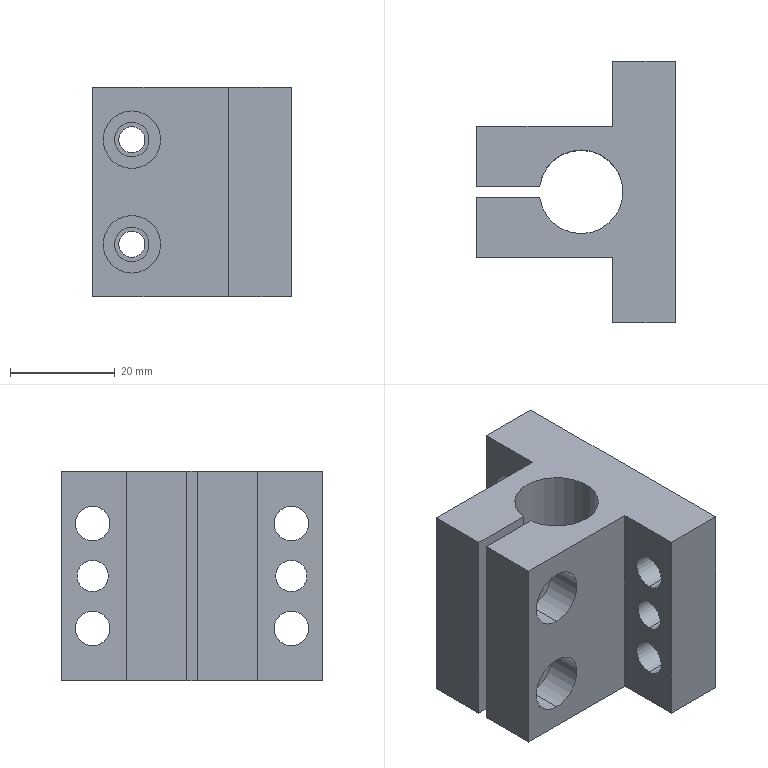Part | STEP file | CLPM16 | 1 solid | 40 faces | box 38 x 50 x 40 mm | volume 36609 mm3 | cylinder 25 | plane 15 | commonest cylinder face diameters 6.6 x12 5 x4 6 x4 11 x4 16 x1
STEP:
#1=CARTESIAN_POINT('',(18.,-19.,17.));
#2=VERTEX_POINT('',#1);
#3=CARTESIAN_POINT('',(18.,-19.,23.));
#4=VERTEX_POINT('',#3);
#5=CARTESIAN_POINT('',(18.,-19.,20.));
#6=DIRECTION('',(-1.,0.,0.));
#7=DIRECTION('',(0.,-1.,0.));
#8=AXIS2_PLACEMENT_3D('',#5,#6,#7);
#9=CIRCLE('',#8,3.);
#10=EDGE_CURVE('',#2,#4,#9,.T.);
#11=ORIENTED_EDGE('',*,*,#10,.F.);
#12=CARTESIAN_POINT('',(6.,-19.,17.));
#13=VERTEX_POINT('',#12);
#14=CARTESIAN_POINT('',(6.,-19.,17.));
#15=DIRECTION('',(-1.,0.,0.));
#16=VECTOR('',#15,1000.);
#17=LINE('',#14,#16);
#18=EDGE_CURVE('',#2,#13,#17,.T.);
#19=ORIENTED_EDGE('',*,*,#18,.T.);
#20=CARTESIAN_POINT('',(6.,-19.,23.));
#21=VERTEX_POINT('',#20);
#22=CARTESIAN_POINT('',(6.,-19.,20.));
#23=DIRECTION('',(-1.,0.,0.));
#24=DIRECTION('',(0.,0.,1.));
#25=AXIS2_PLACEMENT_3D('',#22,#23,#24);
#26=CIRCLE('',#25,3.);
#27=EDGE_CURVE('',#13,#21,#26,.T.);
#28=ORIENTED_EDGE('',*,*,#27,.T.);
#29=CARTESIAN_POINT('',(6.,-19.,23.));
#30=DIRECTION('',(-1.,0.,0.));
#31=VECTOR('',#30,1000.);
#32=LINE('',#29,#31);
#33=EDGE_CURVE('',#4,#21,#32,.T.);
#34=ORIENTED_EDGE('',*,*,#33,.F.);
#35=EDGE_LOOP('',(#11,#19,#28,#34));
#36=FACE_OUTER_BOUND('',#35,.T.);
#37=CARTESIAN_POINT('',(6.,-19.,20.));
#38=DIRECTION('',(-1.,0.,0.));
#39=DIRECTION('',(0.,0.,1.));
#40=AXIS2_PLACEMENT_3D('',#37,#38,#39);
#41=CYLINDRICAL_SURFACE('',#40,3.);
#42=ADVANCED_FACE('',(#36),#41,.F.);
#43=CARTESIAN_POINT('',(18.,19.,17.));
#44=VERTEX_POINT('',#43);
#45=CARTESIAN_POINT('',(18.,19.,23.));
#46=VERTEX_POINT('',#45);
#47=CARTESIAN_POINT('',(18.,19.,20.));
#48=DIRECTION('',(-1.,0.,0.));
#49=DIRECTION('',(0.,-1.,0.));
#50=AXIS2_PLACEMENT_3D('',#47,#48,#49);
#51=CIRCLE('',#50,3.);
#52=EDGE_CURVE('',#44,#46,#51,.T.);
#53=ORIENTED_EDGE('',*,*,#52,.F.);
#54=CARTESIAN_POINT('',(6.,19.,17.));
#55=VERTEX_POINT('',#54);
#56=CARTESIAN_POINT('',(6.,19.,17.));
#57=DIRECTION('',(-1.,0.,0.));
#58=VECTOR('',#57,1000.);
#59=LINE('',#56,#58);
#60=EDGE_CURVE('',#44,#55,#59,.T.);
#61=ORIENTED_EDGE('',*,*,#60,.T.);
#62=CARTESIAN_POINT('',(6.,19.,23.));
#63=VERTEX_POINT('',#62);
#64=CARTESIAN_POINT('',(6.,19.,20.));
#65=DIRECTION('',(-1.,0.,0.));
#66=DIRECTION('',(0.,0.,1.));
#67=AXIS2_PLACEMENT_3D('',#64,#65,#66);
#68=CIRCLE('',#67,3.);
#69=EDGE_CURVE('',#55,#63,#68,.T.);
#70=ORIENTED_EDGE('',*,*,#69,.T.);
#71=CARTESIAN_POINT('',(6.,19.,23.));
#72=DIRECTION('',(-1.,0.,0.));
#73=VECTOR('',#72,1000.);
#74=LINE('',#71,#73);
#75=EDGE_CURVE('',#46,#63,#74,.T.);
#76=ORIENTED_EDGE('',*,*,#75,.F.);
#77=EDGE_LOOP('',(#53,#61,#70,#76));
#78=FACE_OUTER_BOUND('',#77,.T.);
#79=CARTESIAN_POINT('',(6.,19.,20.));
#80=DIRECTION('',(-1.,0.,0.));
#81=DIRECTION('',(0.,0.,1.));
#82=AXIS2_PLACEMENT_3D('',#79,#80,#81);
#83=CYLINDRICAL_SURFACE('',#82,3.);
#84=ADVANCED_FACE('',(#78),#83,.F.);
#85=CARTESIAN_POINT('',(18.,19.,26.7));
#86=VERTEX_POINT('',#85);
#87=CARTESIAN_POINT('',(18.,19.,33.3));
#88=VERTEX_POINT('',#87);
#89=CARTESIAN_POINT('',(18.,19.,30.));
#90=DIRECTION('',(-1.,0.,0.));
#91=DIRECTION('',(0.,-1.,0.));
#92=AXIS2_PLACEMENT_3D('',#89,#90,#91);
#93=CIRCLE('',#92,3.3);
#94=EDGE_CURVE('',#86,#88,#93,.T.);
#95=ORIENTED_EDGE('',*,*,#94,.F.);
#96=CARTESIAN_POINT('',(6.,19.,26.7));
#97=VERTEX_POINT('',#96);
#98=CARTESIAN_POINT('',(6.,19.,26.7));
#99=DIRECTION('',(-1.,0.,0.));
#100=VECTOR('',#99,1000.);
#101=LINE('',#98,#100);
#102=EDGE_CURVE('',#86,#97,#101,.T.);
#103=ORIENTED_EDGE('',*,*,#102,.T.);
#104=CARTESIAN_POINT('',(6.,19.,33.3));
#105=VERTEX_POINT('',#104);
#106=CARTESIAN_POINT('',(6.,19.,30.));
#107=DIRECTION('',(-1.,0.,0.));
#108=DIRECTION('',(0.,0.,1.));
#109=AXIS2_PLACEMENT_3D('',#106,#107,#108);
#110=CIRCLE('',#109,3.3);
#111=EDGE_CURVE('',#97,#105,#110,.T.);
#112=ORIENTED_EDGE('',*,*,#111,.T.);
#113=CARTESIAN_POINT('',(6.,19.,33.3));
#114=DIRECTION('',(-1.,0.,0.));
#115=VECTOR('',#114,1000.);
#116=LINE('',#113,#115);
#117=EDGE_CURVE('',#88,#105,#116,.T.);
#118=ORIENTED_EDGE('',*,*,#117,.F.);
#119=EDGE_LOOP('',(#95,#103,#112,#118));
#120=FACE_OUTER_BOUND('',#119,.T.);
#121=CARTESIAN_POINT('',(6.,19.,30.));
#122=DIRECTION('',(-1.,0.,0.));
#123=DIRECTION('',(0.,0.,1.));
#124=AXIS2_PLACEMENT_3D('',#121,#122,#123);
#125=CYLINDRICAL_SURFACE('',#124,3.3);
#126=ADVANCED_FACE('',(#120),#125,.F.);
#127=CARTESIAN_POINT('',(18.,19.,6.7));
#128=VERTEX_POINT('',#127);
#129=CARTESIAN_POINT('',(18.,19.,13.3));
#130=VERTEX_POINT('',#129);
#131=CARTESIAN_POINT('',(18.,19.,10.));
#132=DIRECTION('',(-1.,0.,0.));
#133=DIRECTION('',(0.,-1.,0.));
#134=AXIS2_PLACEMENT_3D('',#131,#132,#133);
#135=CIRCLE('',#134,3.3);
#136=EDGE_CURVE('',#128,#130,#135,.T.);
#137=ORIENTED_EDGE('',*,*,#136,.F.);
#138=CARTESIAN_POINT('',(6.,19.,6.7));
#139=VERTEX_POINT('',#138);
#140=CARTESIAN_POINT('',(6.,19.,6.7));
#141=DIRECTION('',(-1.,0.,0.));
#142=VECTOR('',#141,1000.);
#143=LINE('',#140,#142);
#144=EDGE_CURVE('',#128,#139,#143,.T.);
#145=ORIENTED_EDGE('',*,*,#144,.T.);
#146=CARTESIAN_POINT('',(6.,19.,13.3));
#147=VERTEX_POINT('',#146);
#148=CARTESIAN_POINT('',(6.,19.,10.));
#149=DIRECTION('',(-1.,0.,0.));
#150=DIRECTION('',(0.,0.,1.));
#151=AXIS2_PLACEMENT_3D('',#148,#149,#150);
#152=CIRCLE('',#151,3.3);
#153=EDGE_CURVE('',#139,#147,#152,.T.);
#154=ORIENTED_EDGE('',*,*,#153,.T.);
#155=CARTESIAN_POINT('',(6.,19.,13.3));
#156=DIRECTION('',(-1.,0.,0.));
#157=VECTOR('',#156,1000.);
#158=LINE('',#155,#157);
#159=EDGE_CURVE('',#130,#147,#158,.T.);
#160=ORIENTED_EDGE('',*,*,#159,.F.);
#161=EDGE_LOOP('',(#137,#145,#154,#160));
#162=FACE_OUTER_BOUND('',#161,.T.);
#163=CARTESIAN_POINT('',(6.,19.,10.));
#164=DIRECTION('',(-1.,0.,0.));
#165=DIRECTION('',(0.,0.,1.));
#166=AXIS2_PLACEMENT_3D('',#163,#164,#165);
#167=CYLINDRICAL_SURFACE('',#166,3.3);
#168=ADVANCED_FACE('',(#162),#167,.F.);
#169=CARTESIAN_POINT('',(18.,-19.,6.7));
#170=VERTEX_POINT('',#169);
#171=CARTESIAN_POINT('',(18.,-19.,13.3));
#172=VERTEX_POINT('',#171);
#173=CARTESIAN_POINT('',(18.,-19.,10.));
#174=DIRECTION('',(-1.,0.,0.));
#175=DIRECTION('',(0.,-1.,0.));
#176=AXIS2_PLACEMENT_3D('',#173,#174,#175);
#177=CIRCLE('',#176,3.3);
#178=EDGE_CURVE('',#170,#172,#177,.T.);
#179=ORIENTED_EDGE('',*,*,#178,.F.);
#180=CARTESIAN_POINT('',(6.,-19.,6.7));
#181=VERTEX_POINT('',#180);
#182=CARTESIAN_POINT('',(6.,-19.,6.7));
#183=DIRECTION('',(-1.,0.,0.));
#184=VECTOR('',#183,1000.);
#185=LINE('',#182,#184);
#186=EDGE_CURVE('',#170,#181,#185,.T.);
#187=ORIENTED_EDGE('',*,*,#186,.T.);
#188=CARTESIAN_POINT('',(6.,-19.,13.3));
#189=VERTEX_POINT('',#188);
#190=CARTESIAN_POINT('',(6.,-19.,10.));
#191=DIRECTION('',(-1.,0.,0.));
#192=DIRECTION('',(0.,0.,1.));
#193=AXIS2_PLACEMENT_3D('',#190,#191,#192);
#194=CIRCLE('',#193,3.3);
#195=EDGE_CURVE('',#181,#189,#194,.T.);
#196=ORIENTED_EDGE('',*,*,#195,.T.);
#197=CARTESIAN_POINT('',(6.,-19.,13.3));
#198=DIRECTION('',(-1.,0.,0.));
#199=VECTOR('',#198,1000.);
#200=LINE('',#197,#199);
#201=EDGE_CURVE('',#172,#189,#200,.T.);
#202=ORIENTED_EDGE('',*,*,#201,.F.);
#203=EDGE_LOOP('',(#179,#187,#196,#202));
#204=FACE_OUTER_BOUND('',#203,.T.);
#205=CARTESIAN_POINT('',(6.,-19.,10.));
#206=DIRECTION('',(-1.,0.,0.));
#207=DIRECTION('',(0.,0.,1.));
#208=AXIS2_PLACEMENT_3D('',#205,#206,#207);
#209=CYLINDRICAL_SURFACE('',#208,3.3);
#210=ADVANCED_FACE('',(#204),#209,.F.);
#211=CARTESIAN_POINT('',(18.,-19.,26.7));
#212=VERTEX_POINT('',#211);
#213=CARTESIAN_POINT('',(18.,-19.,33.3));
#214=VERTEX_POINT('',#213);
#215=CARTESIAN_POINT('',(18.,-19.,30.));
#216=DIRECTION('',(-1.,0.,0.));
#217=DIRECTION('',(0.,-1.,0.));
#218=AXIS2_PLACEMENT_3D('',#215,#216,#217);
#219=CIRCLE('',#218,3.3);
#220=EDGE_CURVE('',#212,#214,#219,.T.);
#221=ORIENTED_EDGE('',*,*,#220,.F.);
#222=CARTESIAN_POINT('',(6.,-19.,26.7));
#223=VERTEX_POINT('',#222);
#224=CARTESIAN_POINT('',(6.,-19.,26.7));
#225=DIRECTION('',(-1.,0.,0.));
#226=VECTOR('',#225,1000.);
#227=LINE('',#224,#226);
#228=EDGE_CURVE('',#212,#223,#227,.T.);
#229=ORIENTED_EDGE('',*,*,#228,.T.);
#230=CARTESIAN_POINT('',(6.,-19.,33.3));
#231=VERTEX_POINT('',#230);
#232=CARTESIAN_POINT('',(6.,-19.,30.));
#233=DIRECTION('',(-1.,0.,0.));
#234=DIRECTION('',(0.,0.,1.));
#235=AXIS2_PLACEMENT_3D('',#232,#233,#234);
#236=CIRCLE('',#235,3.3);
#237=EDGE_CURVE('',#223,#231,#236,.T.);
#238=ORIENTED_EDGE('',*,*,#237,.T.);
#239=CARTESIAN_POINT('',(6.,-19.,33.3));
#240=DIRECTION('',(-1.,0.,0.));
#241=VECTOR('',#240,1000.);
#242=LINE('',#239,#241);
#243=EDGE_CURVE('',#214,#231,#242,.T.);
#244=ORIENTED_EDGE('',*,*,#243,.F.);
#245=EDGE_LOOP('',(#221,#229,#238,#244));
#246=FACE_OUTER_BOUND('',#245,.T.);
#247=CARTESIAN_POINT('',(6.,-19.,30.));
#248=DIRECTION('',(-1.,0.,0.));
#249=DIRECTION('',(0.,0.,1.));
#250=AXIS2_PLACEMENT_3D('',#247,#248,#249);
#251=CYLINDRICAL_SURFACE('',#250,3.3);
#252=ADVANCED_FACE('',(#246),#251,.F.);
#253=CARTESIAN_POINT('',(-12.5,12.5,12.5));
#254=VERTEX_POINT('',#253);
#255=CARTESIAN_POINT('',(-12.5,12.5,7.5));
#256=VERTEX_POINT('',#255);
#257=CARTESIAN_POINT('',(-12.5,12.5,10.));
#258=DIRECTION('',(0.,-1.,0.));
#259=DIRECTION('',(0.,0.,-1.));
#260=AXIS2_PLACEMENT_3D('',#257,#258,#259);
#261=CIRCLE('',#260,2.5);
#262=EDGE_CURVE('',#254,#256,#261,.T.);
#263=ORIENTED_EDGE('',*,*,#262,.F.);
#264=CARTESIAN_POINT('',(-12.5,1.,12.5));
#265=VERTEX_POINT('',#264);
#266=CARTESIAN_POINT('',(-12.5,1.,12.5));
#267=DIRECTION('',(0.,-1.,0.));
#268=VECTOR('',#267,1000.);
#269=LINE('',#266,#268);
#270=EDGE_CURVE('',#254,#265,#269,.T.);
#271=ORIENTED_EDGE('',*,*,#270,.T.);
#272=CARTESIAN_POINT('',(-12.5,1.,7.5));
#273=VERTEX_POINT('',#272);
#274=CARTESIAN_POINT('',(-12.5,1.,10.));
#275=DIRECTION('',(0.,-1.,0.));
#276=DIRECTION('',(0.,0.,-1.));
#277=AXIS2_PLACEMENT_3D('',#274,#275,#276);
#278=CIRCLE('',#277,2.5);
#279=EDGE_CURVE('',#265,#273,#278,.T.);
#280=ORIENTED_EDGE('',*,*,#279,.T.);
#281=CARTESIAN_POINT('',(-12.5,1.,7.5));
#282=DIRECTION('',(0.,-1.,0.));
#283=VECTOR('',#282,1000.);
#284=LINE('',#281,#283);
#285=EDGE_CURVE('',#256,#273,#284,.T.);
#286=ORIENTED_EDGE('',*,*,#285,.F.);
#287=EDGE_LOOP('',(#263,#271,#280,#286));
#288=FACE_OUTER_BOUND('',#287,.T.);
#289=CARTESIAN_POINT('',(-12.5,1.,10.));
#290=DIRECTION('',(0.,-1.,0.));
#291=DIRECTION('',(0.,0.,-1.));
#292=AXIS2_PLACEMENT_3D('',#289,#290,#291);
#293=CYLINDRICAL_SURFACE('',#292,2.5);
#294=ADVANCED_FACE('',(#288),#293,.F.);
#295=CARTESIAN_POINT('',(-12.5,12.5,32.5));
#296=VERTEX_POINT('',#295);
#297=CARTESIAN_POINT('',(-12.5,12.5,27.5));
#298=VERTEX_POINT('',#297);
#299=CARTESIAN_POINT('',(-12.5,12.5,30.));
#300=DIRECTION('',(0.,-1.,0.));
#301=DIRECTION('',(0.,0.,-1.));
#302=AXIS2_PLACEMENT_3D('',#299,#300,#301);
#303=CIRCLE('',#302,2.5);
#304=EDGE_CURVE('',#296,#298,#303,.T.);
#305=ORIENTED_EDGE('',*,*,#304,.F.);
#306=CARTESIAN_POINT('',(-12.5,1.,32.5));
#307=VERTEX_POINT('',#306);
#308=CARTESIAN_POINT('',(-12.5,1.,32.5));
#309=DIRECTION('',(0.,-1.,0.));
#310=VECTOR('',#309,1000.);
#311=LINE('',#308,#310);
#312=EDGE_CURVE('',#296,#307,#311,.T.);
#313=ORIENTED_EDGE('',*,*,#312,.T.);
#314=CARTESIAN_POINT('',(-12.5,1.,27.5));
#315=VERTEX_POINT('',#314);
#316=CARTESIAN_POINT('',(-12.5,1.,30.));
#317=DIRECTION('',(0.,-1.,0.));
#318=DIRECTION('',(0.,0.,-1.));
#319=AXIS2_PLACEMENT_3D('',#316,#317,#318);
#320=CIRCLE('',#319,2.5);
#321=EDGE_CURVE('',#307,#315,#320,.T.);
#322=ORIENTED_EDGE('',*,*,#321,.T.);
#323=CARTESIAN_POINT('',(-12.5,1.,27.5));
#324=DIRECTION('',(0.,-1.,0.));
#325=VECTOR('',#324,1000.);
#326=LINE('',#323,#325);
#327=EDGE_CURVE('',#298,#315,#326,.T.);
#328=ORIENTED_EDGE('',*,*,#327,.F.);
#329=EDGE_LOOP('',(#305,#313,#322,#328));
#330=FACE_OUTER_BOUND('',#329,.T.);
#331=CARTESIAN_POINT('',(-12.5,1.,30.));
#332=DIRECTION('',(0.,-1.,0.));
#333=DIRECTION('',(0.,0.,-1.));
#334=AXIS2_PLACEMENT_3D('',#331,#332,#333);
#335=CYLINDRICAL_SURFACE('',#334,2.5);
#336=ADVANCED_FACE('',(#330),#335,.F.);
#337=CARTESIAN_POINT('',(-12.5,-5.7,15.5));
#338=VERTEX_POINT('',#337);
#339=CARTESIAN_POINT('',(-12.5,-5.7,4.5));
#340=VERTEX_POINT('',#339);
#341=CARTESIAN_POINT('',(-12.5,-5.7,10.));
#342=DIRECTION('',(0.,-1.,0.));
#343=DIRECTION('',(0.,0.,-1.));
#344=AXIS2_PLACEMENT_3D('',#341,#342,#343);
#345=CIRCLE('',#344,5.5);
#346=EDGE_CURVE('',#338,#340,#345,.T.);
#347=ORIENTED_EDGE('',*,*,#346,.F.);
#348=CARTESIAN_POINT('',(-12.5,-12.5,15.5));
#349=VERTEX_POINT('',#348);
#350=CARTESIAN_POINT('',(-12.5,-12.5,15.5));
#351=DIRECTION('',(0.,-1.,0.));
#352=VECTOR('',#351,1000.);
#353=LINE('',#350,#352);
#354=EDGE_CURVE('',#338,#349,#353,.T.);
#355=ORIENTED_EDGE('',*,*,#354,.T.);
#356=CARTESIAN_POINT('',(-12.5,-12.5,4.5));
#357=VERTEX_POINT('',#356);
#358=CARTESIAN_POINT('',(-12.5,-12.5,10.));
#359=DIRECTION('',(0.,-1.,0.));
#360=DIRECTION('',(0.,0.,-1.));
#361=AXIS2_PLACEMENT_3D('',#358,#359,#360);
#362=CIRCLE('',#361,5.5);
#363=EDGE_CURVE('',#349,#357,#362,.T.);
#364=ORIENTED_EDGE('',*,*,#363,.T.);
#365=CARTESIAN_POINT('',(-12.5,-12.5,4.5));
#366=DIRECTION('',(0.,-1.,0.));
#367=VECTOR('',#366,1000.);
#368=LINE('',#365,#367);
#369=EDGE_CURVE('',#340,#357,#368,.T.);
#370=ORIENTED_EDGE('',*,*,#369,.F.);
#371=EDGE_LOOP('',(#347,#355,#364,#370));
#372=FACE_OUTER_BOUND('',#371,.T.);
#373=CARTESIAN_POINT('',(-12.5,-12.5,10.));
#374=DIRECTION('',(0.,-1.,0.));
#375=DIRECTION('',(0.,0.,-1.));
#376=AXIS2_PLACEMENT_3D('',#373,#374,#375);
#377=CYLINDRICAL_SURFACE('',#376,5.5);
#378=ADVANCED_FACE('',(#372),#377,.F.);
#379=CARTESIAN_POINT('',(-12.5,-1.,13.3));
#380=VERTEX_POINT('',#379);
#381=CARTESIAN_POINT('',(-12.5,-1.,6.7));
#382=VERTEX_POINT('',#381);
#383=CARTESIAN_POINT('',(-12.5,-1.,10.));
#384=DIRECTION('',(0.,-1.,0.));
#385=DIRECTION('',(1.,0.,0.));
#386=AXIS2_PLACEMENT_3D('',#383,#384,#385);
#387=CIRCLE('',#386,3.3);
#388=EDGE_CURVE('',#380,#382,#387,.T.);
#389=ORIENTED_EDGE('',*,*,#388,.F.);
#390=CARTESIAN_POINT('',(-12.5,-5.7,13.3));
#391=VERTEX_POINT('',#390);
#392=CARTESIAN_POINT('',(-12.5,-12.5,13.3));
#393=DIRECTION('',(0.,-1.,0.));
#394=VECTOR('',#393,1000.);
#395=LINE('',#392,#394);
#396=EDGE_CURVE('',#380,#391,#395,.T.);
#397=ORIENTED_EDGE('',*,*,#396,.T.);
#398=CARTESIAN_POINT('',(-12.5,-5.7,6.7));
#399=VERTEX_POINT('',#398);
#400=CARTESIAN_POINT('',(-12.5,-5.7,10.));
#401=DIRECTION('',(0.,-1.,0.));
#402=DIRECTION('',(0.,0.,-1.));
#403=AXIS2_PLACEMENT_3D('',#400,#401,#402);
#404=CIRCLE('',#403,3.3);
#405=EDGE_CURVE('',#391,#399,#404,.T.);
#406=ORIENTED_EDGE('',*,*,#405,.T.);
#407=CARTESIAN_POINT('',(-12.5,-12.5,6.7));
#408=DIRECTION('',(0.,-1.,0.));
#409=VECTOR('',#408,1000.);
#410=LINE('',#407,#409);
#411=EDGE_CURVE('',#382,#399,#410,.T.);
#412=ORIENTED_EDGE('',*,*,#411,.F.);
#413=EDGE_LOOP('',(#389,#397,#406,#412));
#414=FACE_OUTER_BOUND('',#413,.T.);
#415=CARTESIAN_POINT('',(-12.5,-12.5,10.));
#416=DIRECTION('',(0.,-1.,0.));
#417=DIRECTION('',(0.,0.,-1.));
#418=AXIS2_PLACEMENT_3D('',#415,#416,#417);
#419=CYLINDRICAL_SURFACE('',#418,3.3);
#420=ADVANCED_FACE('',(#414),#419,.F.);
#421=CARTESIAN_POINT('',(-12.5,-5.7,35.5));
#422=VERTEX_POINT('',#421);
#423=CARTESIAN_POINT('',(-12.5,-5.7,24.5));
#424=VERTEX_POINT('',#423);
#425=CARTESIAN_POINT('',(-12.5,-5.7,30.));
#426=DIRECTION('',(0.,-1.,0.));
#427=DIRECTION('',(0.,0.,-1.));
#428=AXIS2_PLACEMENT_3D('',#425,#426,#427);
#429=CIRCLE('',#428,5.5);
#430=EDGE_CURVE('',#422,#424,#429,.T.);
#431=ORIENTED_EDGE('',*,*,#430,.F.);
#432=CARTESIAN_POINT('',(-12.5,-12.5,35.5));
#433=VERTEX_POINT('',#432);
#434=CARTESIAN_POINT('',(-12.5,-12.5,35.5));
#435=DIRECTION('',(0.,-1.,0.));
#436=VECTOR('',#435,1000.);
#437=LINE('',#434,#436);
#438=EDGE_CURVE('',#422,#433,#437,.T.);
#439=ORIENTED_EDGE('',*,*,#438,.T.);
#440=CARTESIAN_POINT('',(-12.5,-12.5,24.5));
#441=VERTEX_POINT('',#440);
#442=CARTESIAN_POINT('',(-12.5,-12.5,30.));
#443=DIRECTION('',(0.,-1.,0.));
#444=DIRECTION('',(0.,0.,-1.));
#445=AXIS2_PLACEMENT_3D('',#442,#443,#444);
#446=CIRCLE('',#445,5.5);
#447=EDGE_CURVE('',#433,#441,#446,.T.);
#448=ORIENTED_EDGE('',*,*,#447,.T.);
#449=CARTESIAN_POINT('',(-12.5,-12.5,24.5));
#450=DIRECTION('',(0.,-1.,0.));
#451=VECTOR('',#450,1000.);
#452=LINE('',#449,#451);
#453=EDGE_CURVE('',#424,#441,#452,.T.);
#454=ORIENTED_EDGE('',*,*,#453,.F.);
#455=EDGE_LOOP('',(#431,#439,#448,#454));
#456=FACE_OUTER_BOUND('',#455,.T.);
#457=CARTESIAN_POINT('',(-12.5,-12.5,30.));
#458=DIRECTION('',(0.,-1.,0.));
#459=DIRECTION('',(0.,0.,-1.));
#460=AXIS2_PLACEMENT_3D('',#457,#458,#459);
#461=CYLINDRICAL_SURFACE('',#460,5.5);
#462=ADVANCED_FACE('',(#456),#461,.F.);
#463=CARTESIAN_POINT('',(-12.5,-1.,33.3));
#464=VERTEX_POINT('',#463);
#465=CARTESIAN_POINT('',(-12.5,-1.,26.7));
#466=VERTEX_POINT('',#465);
#467=CARTESIAN_POINT('',(-12.5,-1.,30.));
#468=DIRECTION('',(0.,-1.,0.));
#469=DIRECTION('',(1.,0.,0.));
#470=AXIS2_PLACEMENT_3D('',#467,#468,#469);
#471=CIRCLE('',#470,3.3);
#472=EDGE_CURVE('',#464,#466,#471,.T.);
#473=ORIENTED_EDGE('',*,*,#472,.F.);
#474=CARTESIAN_POINT('',(-12.5,-5.7,33.3));
#475=VERTEX_POINT('',#474);
#476=CARTESIAN_POINT('',(-12.5,-12.5,33.3));
#477=DIRECTION('',(0.,-1.,0.));
#478=VECTOR('',#477,1000.);
#479=LINE('',#476,#478);
#480=EDGE_CURVE('',#464,#475,#479,.T.);
#481=ORIENTED_EDGE('',*,*,#480,.T.);
#482=CARTESIAN_POINT('',(-12.5,-5.7,26.7));
#483=VERTEX_POINT('',#482);
#484=CARTESIAN_POINT('',(-12.5,-5.7,30.));
#485=DIRECTION('',(0.,-1.,0.));
#486=DIRECTION('',(0.,0.,-1.));
#487=AXIS2_PLACEMENT_3D('',#484,#485,#486);
#488=CIRCLE('',#487,3.3);
#489=EDGE_CURVE('',#475,#483,#488,.T.);
#490=ORIENTED_EDGE('',*,*,#489,.T.);
#491=CARTESIAN_POINT('',(-12.5,-12.5,26.7));
#492=DIRECTION('',(0.,-1.,0.));
#493=VECTOR('',#492,1000.);
#494=LINE('',#491,#493);
#495=EDGE_CURVE('',#466,#483,#494,.T.);
#496=ORIENTED_EDGE('',*,*,#495,.F.);
#497=EDGE_LOOP('',(#473,#481,#490,#496));
#498=FACE_OUTER_BOUND('',#497,.T.);
#499=CARTESIAN_POINT('',(-12.5,-12.5,30.));
#500=DIRECTION('',(0.,-1.,0.));
#501=DIRECTION('',(0.,0.,-1.));
#502=AXIS2_PLACEMENT_3D('',#499,#500,#501);
#503=CYLINDRICAL_SURFACE('',#502,3.3);
#504=ADVANCED_FACE('',(#498),#503,.F.);
#505=CARTESIAN_POINT('',(-12.5,-12.5,30.));
#506=DIRECTION('',(0.,-1.,0.));
#507=DIRECTION('',(0.,0.,-1.));
#508=AXIS2_PLACEMENT_3D('',#505,#506,#507);
#509=CIRCLE('',#508,5.5);
#510=EDGE_CURVE('',#441,#433,#509,.T.);
#511=ORIENTED_EDGE('',*,*,#510,.F.);
#512=ORIENTED_EDGE('',*,*,#447,.F.);
#513=EDGE_LOOP('',(#511,#512));
#514=FACE_BOUND('',#513,.T.);
#515=CARTESIAN_POINT('',(-20.,-12.5,0.));
#516=VERTEX_POINT('',#515);
#517=CARTESIAN_POINT('',(6.,-12.5,0.));
#518=VERTEX_POINT('',#517);
#519=CARTESIAN_POINT('',(-20.,-12.5,0.));
#520=DIRECTION('',(1.,0.,0.));
#521=VECTOR('',#520,1000.);
#522=LINE('',#519,#521);
#523=EDGE_CURVE('',#516,#518,#522,.T.);
#524=ORIENTED_EDGE('',*,*,#523,.T.);
#525=CARTESIAN_POINT('',(6.,-12.5,40.));
#526=VERTEX_POINT('',#525);
#527=CARTESIAN_POINT('',(6.,-12.5,40.));
#528=DIRECTION('',(0.,0.,-1.));
#529=VECTOR('',#528,1000.);
#530=LINE('',#527,#529);
#531=EDGE_CURVE('',#526,#518,#530,.T.);
#532=ORIENTED_EDGE('',*,*,#531,.F.);
#533=CARTESIAN_POINT('',(-20.,-12.5,40.));
#534=VERTEX_POINT('',#533);
#535=CARTESIAN_POINT('',(-20.,-12.5,40.));
#536=DIRECTION('',(1.,0.,0.));
#537=VECTOR('',#536,1000.);
#538=LINE('',#535,#537);
#539=EDGE_CURVE('',#534,#526,#538,.T.);
#540=ORIENTED_EDGE('',*,*,#539,.F.);
#541=CARTESIAN_POINT('',(-20.,-12.5,40.));
#542=DIRECTION('',(0.,0.,-1.));
#543=VECTOR('',#542,1000.);
#544=LINE('',#541,#543);
#545=EDGE_CURVE('',#534,#516,#544,.T.);
#546=ORIENTED_EDGE('',*,*,#545,.T.);
#547=EDGE_LOOP('',(#524,#532,#540,#546));
#548=FACE_OUTER_BOUND('',#547,.T.);
#549=CARTESIAN_POINT('',(-12.5,-12.5,10.));
#550=DIRECTION('',(0.,-1.,0.));
#551=DIRECTION('',(0.,0.,-1.));
#552=AXIS2_PLACEMENT_3D('',#549,#550,#551);
#553=CIRCLE('',#552,5.5);
#554=EDGE_CURVE('',#357,#349,#553,.T.);
#555=ORIENTED_EDGE('',*,*,#554,.F.);
#556=ORIENTED_EDGE('',*,*,#363,.F.);
#557=EDGE_LOOP('',(#555,#556));
#558=FACE_BOUND('',#557,.T.);
#559=CARTESIAN_POINT('',(-20.,-12.5,40.));
#560=DIRECTION('',(0.,1.,0.));
#561=DIRECTION('',(0.,0.,1.));
#562=AXIS2_PLACEMENT_3D('',#559,#560,#561);
#563=PLANE('',#562);
#564=ADVANCED_FACE('',(#514,#548,#558),#563,.F.);
#565=CARTESIAN_POINT('',(-20.,-1.,0.));
#566=VERTEX_POINT('',#565);
#567=CARTESIAN_POINT('',(-20.,-1.,0.));
#568=DIRECTION('',(0.,-1.,0.));
#569=VECTOR('',#568,1000.);
#570=LINE('',#567,#569);
#571=EDGE_CURVE('',#566,#516,#570,.T.);
#572=ORIENTED_EDGE('',*,*,#571,.T.);
#573=ORIENTED_EDGE('',*,*,#545,.F.);
#574=CARTESIAN_POINT('',(-20.,-1.,40.));
#575=VERTEX_POINT('',#574);
#576=CARTESIAN_POINT('',(-20.,-1.,40.));
#577=DIRECTION('',(0.,-1.,0.));
#578=VECTOR('',#577,1000.);
#579=LINE('',#576,#578);
#580=EDGE_CURVE('',#575,#534,#579,.T.);
#581=ORIENTED_EDGE('',*,*,#580,.F.);
#582=CARTESIAN_POINT('',(-20.,-1.,40.));
#583=DIRECTION('',(0.,0.,-1.));
#584=VECTOR('',#583,1000.);
#585=LINE('',#582,#584);
#586=EDGE_CURVE('',#575,#566,#585,.T.);
#587=ORIENTED_EDGE('',*,*,#586,.T.);
#588=EDGE_LOOP('',(#572,#573,#581,#587));
#589=FACE_OUTER_BOUND('',#588,.T.);
#590=CARTESIAN_POINT('',(-20.,-1.,40.));
#591=DIRECTION('',(1.,0.,0.));
#592=DIRECTION('',(0.,1.,0.));
#593=AXIS2_PLACEMENT_3D('',#590,#591,#592);
#594=PLANE('',#593);
#595=ADVANCED_FACE('',(#589),#594,.F.);
#596=CARTESIAN_POINT('',(6.,-19.,20.));
#597=DIRECTION('',(-1.,0.,0.));
#598=DIRECTION('',(0.,0.,1.));
#599=AXIS2_PLACEMENT_3D('',#596,#597,#598);
#600=CIRCLE('',#599,3.);
#601=EDGE_CURVE('',#21,#13,#600,.T.);
#602=ORIENTED_EDGE('',*,*,#601,.F.);
#603=ORIENTED_EDGE('',*,*,#27,.F.);
#604=EDGE_LOOP('',(#602,#603));
#605=FACE_BOUND('',#604,.T.);
#606=CARTESIAN_POINT('',(6.,-19.,10.));
#607=DIRECTION('',(-1.,0.,0.));
#608=DIRECTION('',(0.,0.,1.));
#609=AXIS2_PLACEMENT_3D('',#606,#607,#608);
#610=CIRCLE('',#609,3.3);
#611=EDGE_CURVE('',#189,#181,#610,.T.);
#612=ORIENTED_EDGE('',*,*,#611,.F.);
#613=ORIENTED_EDGE('',*,*,#195,.F.);
#614=EDGE_LOOP('',(#612,#613));
#615=FACE_BOUND('',#614,.T.);
#616=CARTESIAN_POINT('',(6.,-19.,30.));
#617=DIRECTION('',(-1.,0.,0.));
#618=DIRECTION('',(0.,0.,1.));
#619=AXIS2_PLACEMENT_3D('',#616,#617,#618);
#620=CIRCLE('',#619,3.3);
#621=EDGE_CURVE('',#231,#223,#620,.T.);
#622=ORIENTED_EDGE('',*,*,#621,.F.);
#623=ORIENTED_EDGE('',*,*,#237,.F.);
#624=EDGE_LOOP('',(#622,#623));
#625=FACE_BOUND('',#624,.T.);
#626=CARTESIAN_POINT('',(6.,-25.,0.));
#627=VERTEX_POINT('',#626);
#628=CARTESIAN_POINT('',(6.,-12.5,0.));
#629=DIRECTION('',(0.,-1.,0.));
#630=VECTOR('',#629,1000.);
#631=LINE('',#628,#630);
#632=EDGE_CURVE('',#518,#627,#631,.T.);
#633=ORIENTED_EDGE('',*,*,#632,.T.);
#634=CARTESIAN_POINT('',(6.,-25.,40.));
#635=VERTEX_POINT('',#634);
#636=CARTESIAN_POINT('',(6.,-25.,40.));
#637=DIRECTION('',(0.,0.,-1.));
#638=VECTOR('',#637,1000.);
#639=LINE('',#636,#638);
#640=EDGE_CURVE('',#635,#627,#639,.T.);
#641=ORIENTED_EDGE('',*,*,#640,.F.);
#642=CARTESIAN_POINT('',(6.,-12.5,40.));
#643=DIRECTION('',(0.,-1.,0.));
#644=VECTOR('',#643,1000.);
#645=LINE('',#642,#644);
#646=EDGE_CURVE('',#526,#635,#645,.T.);
#647=ORIENTED_EDGE('',*,*,#646,.F.);
#648=ORIENTED_EDGE('',*,*,#531,.T.);
#649=EDGE_LOOP('',(#633,#641,#647,#648));
#650=FACE_OUTER_BOUND('',#649,.T.);
#651=CARTESIAN_POINT('',(6.,-12.5,40.));
#652=DIRECTION('',(1.,0.,0.));
#653=DIRECTION('',(0.,1.,0.));
#654=AXIS2_PLACEMENT_3D('',#651,#652,#653);
#655=PLANE('',#654);
#656=ADVANCED_FACE('',(#605,#615,#625,#650),#655,.F.);
#657=CARTESIAN_POINT('',(18.,-25.,0.));
#658=VERTEX_POINT('',#657);
#659=CARTESIAN_POINT('',(6.,-25.,0.));
#660=DIRECTION('',(1.,0.,0.));
#661=VECTOR('',#660,1000.);
#662=LINE('',#659,#661);
#663=EDGE_CURVE('',#627,#658,#662,.T.);
#664=ORIENTED_EDGE('',*,*,#663,.T.);
#665=CARTESIAN_POINT('',(18.,-25.,40.));
#666=VERTEX_POINT('',#665);
#667=CARTESIAN_POINT('',(18.,-25.,40.));
#668=DIRECTION('',(0.,0.,-1.));
#669=VECTOR('',#668,1000.);
#670=LINE('',#667,#669);
#671=EDGE_CURVE('',#666,#658,#670,.T.);
#672=ORIENTED_EDGE('',*,*,#671,.F.);
#673=CARTESIAN_POINT('',(6.,-25.,40.));
#674=DIRECTION('',(1.,0.,0.));
#675=VECTOR('',#674,1000.);
#676=LINE('',#673,#675);
#677=EDGE_CURVE('',#635,#666,#676,.T.);
#678=ORIENTED_EDGE('',*,*,#677,.F.);
#679=ORIENTED_EDGE('',*,*,#640,.T.);
#680=EDGE_LOOP('',(#664,#672,#678,#679));
#681=FACE_OUTER_BOUND('',#680,.T.);
#682=CARTESIAN_POINT('',(6.,-25.,40.));
#683=DIRECTION('',(0.,1.,0.));
#684=DIRECTION('',(0.,0.,1.));
#685=AXIS2_PLACEMENT_3D('',#682,#683,#684);
#686=PLANE('',#685);
#687=ADVANCED_FACE('',(#681),#686,.F.);
#688=CARTESIAN_POINT('',(18.,-19.,20.));
#689=DIRECTION('',(-1.,0.,0.));
#690=DIRECTION('',(0.,-1.,0.));
#691=AXIS2_PLACEMENT_3D('',#688,#689,#690);
#692=CIRCLE('',#691,3.);
#693=EDGE_CURVE('',#4,#2,#692,.T.);
#694=ORIENTED_EDGE('',*,*,#693,.T.);
#695=ORIENTED_EDGE('',*,*,#10,.T.);
#696=EDGE_LOOP('',(#694,#695));
#697=FACE_BOUND('',#696,.T.);
#698=CARTESIAN_POINT('',(18.,19.,20.));
#699=DIRECTION('',(-1.,0.,0.));
#700=DIRECTION('',(0.,-1.,0.));
#701=AXIS2_PLACEMENT_3D('',#698,#699,#700);
#702=CIRCLE('',#701,3.);
#703=EDGE_CURVE('',#46,#44,#702,.T.);
#704=ORIENTED_EDGE('',*,*,#703,.T.);
#705=ORIENTED_EDGE('',*,*,#52,.T.);
#706=EDGE_LOOP('',(#704,#705));
#707=FACE_BOUND('',#706,.T.);
#708=CARTESIAN_POINT('',(18.,19.,30.));
#709=DIRECTION('',(-1.,0.,0.));
#710=DIRECTION('',(0.,-1.,0.));
#711=AXIS2_PLACEMENT_3D('',#708,#709,#710);
#712=CIRCLE('',#711,3.3);
#713=EDGE_CURVE('',#88,#86,#712,.T.);
#714=ORIENTED_EDGE('',*,*,#713,.T.);
#715=ORIENTED_EDGE('',*,*,#94,.T.);
#716=EDGE_LOOP('',(#714,#715));
#717=FACE_BOUND('',#716,.T.);
#718=CARTESIAN_POINT('',(18.,19.,10.));
#719=DIRECTION('',(-1.,0.,0.));
#720=DIRECTION('',(0.,-1.,0.));
#721=AXIS2_PLACEMENT_3D('',#718,#719,#720);
#722=CIRCLE('',#721,3.3);
#723=EDGE_CURVE('',#130,#128,#722,.T.);
#724=ORIENTED_EDGE('',*,*,#723,.T.);
#725=ORIENTED_EDGE('',*,*,#136,.T.);
#726=EDGE_LOOP('',(#724,#725));
#727=FACE_BOUND('',#726,.T.);
#728=CARTESIAN_POINT('',(18.,-19.,10.));
#729=DIRECTION('',(-1.,0.,0.));
#730=DIRECTION('',(0.,-1.,0.));
#731=AXIS2_PLACEMENT_3D('',#728,#729,#730);
#732=CIRCLE('',#731,3.3);
#733=EDGE_CURVE('',#172,#170,#732,.T.);
#734=ORIENTED_EDGE('',*,*,#733,.T.);
#735=ORIENTED_EDGE('',*,*,#178,.T.);
#736=EDGE_LOOP('',(#734,#735));
#737=FACE_BOUND('',#736,.T.);
#738=CARTESIAN_POINT('',(18.,-19.,30.));
#739=DIRECTION('',(-1.,0.,0.));
#740=DIRECTION('',(0.,-1.,0.));
#741=AXIS2_PLACEMENT_3D('',#738,#739,#740);
#742=CIRCLE('',#741,3.3);
#743=EDGE_CURVE('',#214,#212,#742,.T.);
#744=ORIENTED_EDGE('',*,*,#743,.T.);
#745=ORIENTED_EDGE('',*,*,#220,.T.);
#746=EDGE_LOOP('',(#744,#745));
#747=FACE_BOUND('',#746,.T.);
#748=CARTESIAN_POINT('',(18.,25.,0.));
#749=VERTEX_POINT('',#748);
#750=CARTESIAN_POINT('',(18.,25.,0.));
#751=DIRECTION('',(0.,1.,0.));
#752=VECTOR('',#751,1000.);
#753=LINE('',#750,#752);
#754=EDGE_CURVE('',#658,#749,#753,.T.);
#755=ORIENTED_EDGE('',*,*,#754,.T.);
#756=CARTESIAN_POINT('',(18.,25.,40.));
#757=VERTEX_POINT('',#756);
#758=CARTESIAN_POINT('',(18.,25.,40.));
#759=DIRECTION('',(0.,0.,-1.));
#760=VECTOR('',#759,1000.);
#761=LINE('',#758,#760);
#762=EDGE_CURVE('',#757,#749,#761,.T.);
#763=ORIENTED_EDGE('',*,*,#762,.F.);
#764=CARTESIAN_POINT('',(18.,25.,40.));
#765=DIRECTION('',(0.,1.,0.));
#766=VECTOR('',#765,1000.);
#767=LINE('',#764,#766);
#768=EDGE_CURVE('',#666,#757,#767,.T.);
#769=ORIENTED_EDGE('',*,*,#768,.F.);
#770=ORIENTED_EDGE('',*,*,#671,.T.);
#771=EDGE_LOOP('',(#755,#763,#769,#770));
#772=FACE_OUTER_BOUND('',#771,.T.);
#773=CARTESIAN_POINT('',(18.,25.,40.));
#774=DIRECTION('',(-1.,0.,0.));
#775=DIRECTION('',(0.,-1.,0.));
#776=AXIS2_PLACEMENT_3D('',#773,#774,#775);
#777=PLANE('',#776);
#778=ADVANCED_FACE('',(#697,#707,#717,#727,#737,#747,#772),#777,.F.);
#779=CARTESIAN_POINT('',(6.,25.,0.));
#780=VERTEX_POINT('',#779);
#781=CARTESIAN_POINT('',(6.,25.,0.));
#782=DIRECTION('',(-1.,0.,0.));
#783=VECTOR('',#782,1000.);
#784=LINE('',#781,#783);
#785=EDGE_CURVE('',#749,#780,#784,.T.);
#786=ORIENTED_EDGE('',*,*,#785,.T.);
#787=CARTESIAN_POINT('',(6.,25.,40.));
#788=VERTEX_POINT('',#787);
#789=CARTESIAN_POINT('',(6.,25.,40.));
#790=DIRECTION('',(0.,0.,-1.));
#791=VECTOR('',#790,1000.);
#792=LINE('',#789,#791);
#793=EDGE_CURVE('',#788,#780,#792,.T.);
#794=ORIENTED_EDGE('',*,*,#793,.F.);
#795=CARTESIAN_POINT('',(6.,25.,40.));
#796=DIRECTION('',(-1.,0.,0.));
#797=VECTOR('',#796,1000.);
#798=LINE('',#795,#797);
#799=EDGE_CURVE('',#757,#788,#798,.T.);
#800=ORIENTED_EDGE('',*,*,#799,.F.);
#801=ORIENTED_EDGE('',*,*,#762,.T.);
#802=EDGE_LOOP('',(#786,#794,#800,#801));
#803=FACE_OUTER_BOUND('',#802,.T.);
#804=CARTESIAN_POINT('',(6.,25.,40.));
#805=DIRECTION('',(0.,-1.,0.));
#806=DIRECTION('',(0.,0.,-1.));
#807=AXIS2_PLACEMENT_3D('',#804,#805,#806);
#808=PLANE('',#807);
#809=ADVANCED_FACE('',(#803),#808,.F.);
#810=CARTESIAN_POINT('',(6.,19.,20.));
#811=DIRECTION('',(-1.,0.,0.));
#812=DIRECTION('',(0.,0.,1.));
#813=AXIS2_PLACEMENT_3D('',#810,#811,#812);
#814=CIRCLE('',#813,3.);
#815=EDGE_CURVE('',#63,#55,#814,.T.);
#816=ORIENTED_EDGE('',*,*,#815,.F.);
#817=ORIENTED_EDGE('',*,*,#69,.F.);
#818=EDGE_LOOP('',(#816,#817));
#819=FACE_BOUND('',#818,.T.);
#820=CARTESIAN_POINT('',(6.,19.,30.));
#821=DIRECTION('',(-1.,0.,0.));
#822=DIRECTION('',(0.,0.,1.));
#823=AXIS2_PLACEMENT_3D('',#820,#821,#822);
#824=CIRCLE('',#823,3.3);
#825=EDGE_CURVE('',#105,#97,#824,.T.);
#826=ORIENTED_EDGE('',*,*,#825,.F.);
#827=ORIENTED_EDGE('',*,*,#111,.F.);
#828=EDGE_LOOP('',(#826,#827));
#829=FACE_BOUND('',#828,.T.);
#830=CARTESIAN_POINT('',(6.,19.,10.));
#831=DIRECTION('',(-1.,0.,0.));
#832=DIRECTION('',(0.,0.,1.));
#833=AXIS2_PLACEMENT_3D('',#830,#831,#832);
#834=CIRCLE('',#833,3.3);
#835=EDGE_CURVE('',#147,#139,#834,.T.);
#836=ORIENTED_EDGE('',*,*,#835,.F.);
#837=ORIENTED_EDGE('',*,*,#153,.F.);
#838=EDGE_LOOP('',(#836,#837));
#839=FACE_BOUND('',#838,.T.);
#840=CARTESIAN_POINT('',(6.,12.5,0.));
#841=VERTEX_POINT('',#840);
#842=CARTESIAN_POINT('',(6.,12.5,0.));
#843=DIRECTION('',(0.,-1.,0.));
#844=VECTOR('',#843,1000.);
#845=LINE('',#842,#844);
#846=EDGE_CURVE('',#780,#841,#845,.T.);
#847=ORIENTED_EDGE('',*,*,#846,.T.);
#848=CARTESIAN_POINT('',(6.,12.5,40.));
#849=VERTEX_POINT('',#848);
#850=CARTESIAN_POINT('',(6.,12.5,40.));
#851=DIRECTION('',(0.,0.,-1.));
#852=VECTOR('',#851,1000.);
#853=LINE('',#850,#852);
#854=EDGE_CURVE('',#849,#841,#853,.T.);
#855=ORIENTED_EDGE('',*,*,#854,.F.);
#856=CARTESIAN_POINT('',(6.,12.5,40.));
#857=DIRECTION('',(0.,-1.,0.));
#858=VECTOR('',#857,1000.);
#859=LINE('',#856,#858);
#860=EDGE_CURVE('',#788,#849,#859,.T.);
#861=ORIENTED_EDGE('',*,*,#860,.F.);
#862=ORIENTED_EDGE('',*,*,#793,.T.);
#863=EDGE_LOOP('',(#847,#855,#861,#862));
#864=FACE_OUTER_BOUND('',#863,.T.);
#865=CARTESIAN_POINT('',(6.,12.5,40.));
#866=DIRECTION('',(1.,0.,0.));
#867=DIRECTION('',(0.,0.,-1.));
#868=AXIS2_PLACEMENT_3D('',#865,#866,#867);
#869=PLANE('',#868);
#870=ADVANCED_FACE('',(#819,#829,#839,#864),#869,.F.);
#871=CARTESIAN_POINT('',(-12.5,12.5,10.));
#872=DIRECTION('',(0.,-1.,0.));
#873=DIRECTION('',(0.,0.,-1.));
#874=AXIS2_PLACEMENT_3D('',#871,#872,#873);
#875=CIRCLE('',#874,2.5);
#876=EDGE_CURVE('',#256,#254,#875,.T.);
#877=ORIENTED_EDGE('',*,*,#876,.T.);
#878=ORIENTED_EDGE('',*,*,#262,.T.);
#879=EDGE_LOOP('',(#877,#878));
#880=FACE_BOUND('',#879,.T.);
#881=CARTESIAN_POINT('',(-12.5,12.5,30.));
#882=DIRECTION('',(0.,-1.,0.));
#883=DIRECTION('',(0.,0.,-1.));
#884=AXIS2_PLACEMENT_3D('',#881,#882,#883);
#885=CIRCLE('',#884,2.5);
#886=EDGE_CURVE('',#298,#296,#885,.T.);
#887=ORIENTED_EDGE('',*,*,#886,.T.);
#888=ORIENTED_EDGE('',*,*,#304,.T.);
#889=EDGE_LOOP('',(#887,#888));
#890=FACE_BOUND('',#889,.T.);
#891=CARTESIAN_POINT('',(-20.,12.5,0.));
#892=VERTEX_POINT('',#891);
#893=CARTESIAN_POINT('',(-20.,12.5,0.));
#894=DIRECTION('',(-1.,0.,0.));
#895=VECTOR('',#894,1000.);
#896=LINE('',#893,#895);
#897=EDGE_CURVE('',#841,#892,#896,.T.);
#898=ORIENTED_EDGE('',*,*,#897,.T.);
#899=CARTESIAN_POINT('',(-20.,12.5,40.));
#900=VERTEX_POINT('',#899);
#901=CARTESIAN_POINT('',(-20.,12.5,40.));
#902=DIRECTION('',(0.,0.,-1.));
#903=VECTOR('',#902,1000.);
#904=LINE('',#901,#903);
#905=EDGE_CURVE('',#900,#892,#904,.T.);
#906=ORIENTED_EDGE('',*,*,#905,.F.);
#907=CARTESIAN_POINT('',(-20.,12.5,40.));
#908=DIRECTION('',(-1.,0.,0.));
#909=VECTOR('',#908,1000.);
#910=LINE('',#907,#909);
#911=EDGE_CURVE('',#849,#900,#910,.T.);
#912=ORIENTED_EDGE('',*,*,#911,.F.);
#913=ORIENTED_EDGE('',*,*,#854,.T.);
#914=EDGE_LOOP('',(#898,#906,#912,#913));
#915=FACE_OUTER_BOUND('',#914,.T.);
#916=CARTESIAN_POINT('',(-20.,12.5,40.));
#917=DIRECTION('',(0.,-1.,0.));
#918=DIRECTION('',(0.,0.,-1.));
#919=AXIS2_PLACEMENT_3D('',#916,#917,#918);
#920=PLANE('',#919);
#921=ADVANCED_FACE('',(#880,#890,#915),#920,.F.);
#922=CARTESIAN_POINT('',(-20.,1.,0.));
#923=VERTEX_POINT('',#922);
#924=CARTESIAN_POINT('',(-20.,12.5,0.));
#925=DIRECTION('',(0.,-1.,0.));
#926=VECTOR('',#925,1000.);
#927=LINE('',#924,#926);
#928=EDGE_CURVE('',#892,#923,#927,.T.);
#929=ORIENTED_EDGE('',*,*,#928,.T.);
#930=CARTESIAN_POINT('',(-20.,1.,40.));
#931=VERTEX_POINT('',#930);
#932=CARTESIAN_POINT('',(-20.,1.,40.));
#933=DIRECTION('',(0.,0.,-1.));
#934=VECTOR('',#933,1000.);
#935=LINE('',#932,#934);
#936=EDGE_CURVE('',#931,#923,#935,.T.);
#937=ORIENTED_EDGE('',*,*,#936,.F.);
#938=CARTESIAN_POINT('',(-20.,12.5,40.));
#939=DIRECTION('',(0.,-1.,0.));
#940=VECTOR('',#939,1000.);
#941=LINE('',#938,#940);
#942=EDGE_CURVE('',#900,#931,#941,.T.);
#943=ORIENTED_EDGE('',*,*,#942,.F.);
#944=ORIENTED_EDGE('',*,*,#905,.T.);
#945=EDGE_LOOP('',(#929,#937,#943,#944));
#946=FACE_OUTER_BOUND('',#945,.T.);
#947=CARTESIAN_POINT('',(-20.,12.5,40.));
#948=DIRECTION('',(1.,0.,0.));
#949=DIRECTION('',(0.,1.,0.));
#950=AXIS2_PLACEMENT_3D('',#947,#948,#949);
#951=PLANE('',#950);
#952=ADVANCED_FACE('',(#946),#951,.F.);
#953=CARTESIAN_POINT('',(-12.5,1.,10.));
#954=DIRECTION('',(0.,-1.,0.));
#955=DIRECTION('',(0.,0.,-1.));
#956=AXIS2_PLACEMENT_3D('',#953,#954,#955);
#957=CIRCLE('',#956,2.5);
#958=EDGE_CURVE('',#273,#265,#957,.T.);
#959=ORIENTED_EDGE('',*,*,#958,.F.);
#960=ORIENTED_EDGE('',*,*,#279,.F.);
#961=EDGE_LOOP('',(#959,#960));
#962=FACE_BOUND('',#961,.T.);
#963=CARTESIAN_POINT('',(-12.5,1.,30.));
#964=DIRECTION('',(0.,-1.,0.));
#965=DIRECTION('',(0.,0.,-1.));
#966=AXIS2_PLACEMENT_3D('',#963,#964,#965);
#967=CIRCLE('',#966,2.5);
#968=EDGE_CURVE('',#315,#307,#967,.T.);
#969=ORIENTED_EDGE('',*,*,#968,.F.);
#970=ORIENTED_EDGE('',*,*,#321,.F.);
#971=EDGE_LOOP('',(#969,#970));
#972=FACE_BOUND('',#971,.T.);
#973=CARTESIAN_POINT('',(-7.937,1.,0.));
#974=VERTEX_POINT('',#973);
#975=CARTESIAN_POINT('',(-20.,1.,0.));
#976=DIRECTION('',(1.,0.,0.));
#977=VECTOR('',#976,1000.);
#978=LINE('',#975,#977);
#979=EDGE_CURVE('',#923,#974,#978,.T.);
#980=ORIENTED_EDGE('',*,*,#979,.T.);
#981=CARTESIAN_POINT('',(-7.937,1.,40.));
#982=VERTEX_POINT('',#981);
#983=CARTESIAN_POINT('',(-7.937,1.,40.));
#984=DIRECTION('',(0.,0.,-1.));
#985=VECTOR('',#984,1000.);
#986=LINE('',#983,#985);
#987=EDGE_CURVE('',#982,#974,#986,.T.);
#988=ORIENTED_EDGE('',*,*,#987,.F.);
#989=CARTESIAN_POINT('',(-20.,1.,40.));
#990=DIRECTION('',(1.,0.,0.));
#991=VECTOR('',#990,1000.);
#992=LINE('',#989,#991);
#993=EDGE_CURVE('',#931,#982,#992,.T.);
#994=ORIENTED_EDGE('',*,*,#993,.F.);
#995=ORIENTED_EDGE('',*,*,#936,.T.);
#996=EDGE_LOOP('',(#980,#988,#994,#995));
#997=FACE_OUTER_BOUND('',#996,.T.);
#998=CARTESIAN_POINT('',(-20.,1.,40.));
#999=DIRECTION('',(0.,1.,0.));
#1000=DIRECTION('',(-1.,0.,0.));
#1001=AXIS2_PLACEMENT_3D('',#998,#999,#1000);
#1002=PLANE('',#1001);
#1003=ADVANCED_FACE('',(#962,#972,#997),#1002,.F.);
#1004=CARTESIAN_POINT('',(-7.937,-1.,0.));
#1005=VERTEX_POINT('',#1004);
#1006=CARTESIAN_POINT('',(0.,0.,0.));
#1007=DIRECTION('',(0.,0.,-1.));
#1008=DIRECTION('',(1.,0.,0.));
#1009=AXIS2_PLACEMENT_3D('',#1006,#1007,#1008);
#1010=CIRCLE('',#1009,8.);
#1011=EDGE_CURVE('',#974,#1005,#1010,.T.);
#1012=ORIENTED_EDGE('',*,*,#1011,.T.);
#1013=CARTESIAN_POINT('',(-7.937,-1.,40.));
#1014=VERTEX_POINT('',#1013);
#1015=CARTESIAN_POINT('',(-7.937,-1.,40.));
#1016=DIRECTION('',(0.,0.,-1.));
#1017=VECTOR('',#1016,1000.);
#1018=LINE('',#1015,#1017);
#1019=EDGE_CURVE('',#1014,#1005,#1018,.T.);
#1020=ORIENTED_EDGE('',*,*,#1019,.F.);
#1021=CARTESIAN_POINT('',(0.,0.,40.));
#1022=DIRECTION('',(0.,0.,-1.));
#1023=DIRECTION('',(1.,0.,0.));
#1024=AXIS2_PLACEMENT_3D('',#1021,#1022,#1023);
#1025=CIRCLE('',#1024,8.);
#1026=EDGE_CURVE('',#982,#1014,#1025,.T.);
#1027=ORIENTED_EDGE('',*,*,#1026,.F.);
#1028=ORIENTED_EDGE('',*,*,#987,.T.);
#1029=EDGE_LOOP('',(#1012,#1020,#1027,#1028));
#1030=FACE_OUTER_BOUND('',#1029,.T.);
#1031=CARTESIAN_POINT('',(0.,0.,40.));
#1032=DIRECTION('',(0.,0.,-1.));
#1033=DIRECTION('',(-1.,0.,0.));
#1034=AXIS2_PLACEMENT_3D('',#1031,#1032,#1033);
#1035=CYLINDRICAL_SURFACE('',#1034,8.);
#1036=ADVANCED_FACE('',(#1030),#1035,.F.);
#1037=CARTESIAN_POINT('',(-12.5,-1.,10.));
#1038=DIRECTION('',(0.,-1.,0.));
#1039=DIRECTION('',(1.,0.,0.));
#1040=AXIS2_PLACEMENT_3D('',#1037,#1038,#1039);
#1041=CIRCLE('',#1040,3.3);
#1042=EDGE_CURVE('',#382,#380,#1041,.T.);
#1043=ORIENTED_EDGE('',*,*,#1042,.T.);
#1044=ORIENTED_EDGE('',*,*,#388,.T.);
#1045=EDGE_LOOP('',(#1043,#1044));
#1046=FACE_BOUND('',#1045,.T.);
#1047=CARTESIAN_POINT('',(-12.5,-1.,30.));
#1048=DIRECTION('',(0.,-1.,0.));
#1049=DIRECTION('',(1.,0.,0.));
#1050=AXIS2_PLACEMENT_3D('',#1047,#1048,#1049);
#1051=CIRCLE('',#1050,3.3);
#1052=EDGE_CURVE('',#466,#464,#1051,.T.);
#1053=ORIENTED_EDGE('',*,*,#1052,.T.);
#1054=ORIENTED_EDGE('',*,*,#472,.T.);
#1055=EDGE_LOOP('',(#1053,#1054));
#1056=FACE_BOUND('',#1055,.T.);
#1057=CARTESIAN_POINT('',(-20.,-1.,0.));
#1058=DIRECTION('',(-1.,0.,0.));
#1059=VECTOR('',#1058,1000.);
#1060=LINE('',#1057,#1059);
#1061=EDGE_CURVE('',#1005,#566,#1060,.T.);
#1062=ORIENTED_EDGE('',*,*,#1061,.T.);
#1063=ORIENTED_EDGE('',*,*,#586,.F.);
#1064=CARTESIAN_POINT('',(-20.,-1.,40.));
#1065=DIRECTION('',(-1.,0.,0.));
#1066=VECTOR('',#1065,1000.);
#1067=LINE('',#1064,#1066);
#1068=EDGE_CURVE('',#1014,#575,#1067,.T.);
#1069=ORIENTED_EDGE('',*,*,#1068,.F.);
#1070=ORIENTED_EDGE('',*,*,#1019,.T.);
#1071=EDGE_LOOP('',(#1062,#1063,#1069,#1070));
#1072=FACE_OUTER_BOUND('',#1071,.T.);
#1073=CARTESIAN_POINT('',(-20.,-1.,40.));
#1074=DIRECTION('',(0.,-1.,0.));
#1075=DIRECTION('',(1.,0.,0.));
#1076=AXIS2_PLACEMENT_3D('',#1073,#1074,#1075);
#1077=PLANE('',#1076);
#1078=ADVANCED_FACE('',(#1046,#1056,#1072),#1077,.F.);
#1079=ORIENTED_EDGE('',*,*,#580,.T.);
#1080=ORIENTED_EDGE('',*,*,#539,.T.);
#1081=ORIENTED_EDGE('',*,*,#646,.T.);
#1082=ORIENTED_EDGE('',*,*,#677,.T.);
#1083=ORIENTED_EDGE('',*,*,#768,.T.);
#1084=ORIENTED_EDGE('',*,*,#799,.T.);
#1085=ORIENTED_EDGE('',*,*,#860,.T.);
#1086=ORIENTED_EDGE('',*,*,#911,.T.);
#1087=ORIENTED_EDGE('',*,*,#942,.T.);
#1088=ORIENTED_EDGE('',*,*,#993,.T.);
#1089=ORIENTED_EDGE('',*,*,#1026,.T.);
#1090=ORIENTED_EDGE('',*,*,#1068,.T.);
#1091=EDGE_LOOP('',(#1079,#1080,#1081,#1082,#1083,#1084,#1085,#1086,#1087,#1088,#1089,#1090));
#1092=FACE_OUTER_BOUND('',#1091,.T.);
#1093=CARTESIAN_POINT('',(0.,0.,40.));
#1094=DIRECTION('',(0.,0.,1.));
#1095=DIRECTION('',(1.,0.,0.));
#1096=AXIS2_PLACEMENT_3D('',#1093,#1094,#1095);
#1097=PLANE('',#1096);
#1098=ADVANCED_FACE('',(#1092),#1097,.T.);
#1099=ORIENTED_EDGE('',*,*,#571,.F.);
#1100=ORIENTED_EDGE('',*,*,#1061,.F.);
#1101=ORIENTED_EDGE('',*,*,#1011,.F.);
#1102=ORIENTED_EDGE('',*,*,#979,.F.);
#1103=ORIENTED_EDGE('',*,*,#928,.F.);
#1104=ORIENTED_EDGE('',*,*,#897,.F.);
#1105=ORIENTED_EDGE('',*,*,#846,.F.);
#1106=ORIENTED_EDGE('',*,*,#785,.F.);
#1107=ORIENTED_EDGE('',*,*,#754,.F.);
#1108=ORIENTED_EDGE('',*,*,#663,.F.);
#1109=ORIENTED_EDGE('',*,*,#632,.F.);
#1110=ORIENTED_EDGE('',*,*,#523,.F.);
#1111=EDGE_LOOP('',(#1099,#1100,#1101,#1102,#1103,#1104,#1105,#1106,#1107,#1108,#1109,#1110));
#1112=FACE_OUTER_BOUND('',#1111,.T.);
#1113=CARTESIAN_POINT('',(0.,0.,0.));
#1114=DIRECTION('',(0.,0.,1.));
#1115=DIRECTION('',(1.,0.,0.));
#1116=AXIS2_PLACEMENT_3D('',#1113,#1114,#1115);
#1117=PLANE('',#1116);
#1118=ADVANCED_FACE('',(#1112),#1117,.F.);
#1119=ORIENTED_EDGE('',*,*,#480,.F.);
#1120=ORIENTED_EDGE('',*,*,#1052,.F.);
#1121=ORIENTED_EDGE('',*,*,#495,.T.);
#1122=CARTESIAN_POINT('',(-12.5,-5.7,30.));
#1123=DIRECTION('',(0.,-1.,0.));
#1124=DIRECTION('',(0.,0.,-1.));
#1125=AXIS2_PLACEMENT_3D('',#1122,#1123,#1124);
#1126=CIRCLE('',#1125,3.3);
#1127=EDGE_CURVE('',#483,#475,#1126,.T.);
#1128=ORIENTED_EDGE('',*,*,#1127,.T.);
#1129=EDGE_LOOP('',(#1119,#1120,#1121,#1128));
#1130=FACE_OUTER_BOUND('',#1129,.T.);
#1131=CARTESIAN_POINT('',(-12.5,-12.5,30.));
#1132=DIRECTION('',(0.,-1.,0.));
#1133=DIRECTION('',(0.,0.,-1.));
#1134=AXIS2_PLACEMENT_3D('',#1131,#1132,#1133);
#1135=CYLINDRICAL_SURFACE('',#1134,3.3);
#1136=ADVANCED_FACE('',(#1130),#1135,.F.);
#1137=ORIENTED_EDGE('',*,*,#1127,.F.);
#1138=ORIENTED_EDGE('',*,*,#489,.F.);
#1139=EDGE_LOOP('',(#1137,#1138));
#1140=FACE_BOUND('',#1139,.T.);
#1141=CARTESIAN_POINT('',(-12.5,-5.7,30.));
#1142=DIRECTION('',(0.,-1.,0.));
#1143=DIRECTION('',(0.,0.,-1.));
#1144=AXIS2_PLACEMENT_3D('',#1141,#1142,#1143);
#1145=CIRCLE('',#1144,5.5);
#1146=EDGE_CURVE('',#424,#422,#1145,.T.);
#1147=ORIENTED_EDGE('',*,*,#1146,.T.);
#1148=ORIENTED_EDGE('',*,*,#430,.T.);
#1149=EDGE_LOOP('',(#1147,#1148));
#1150=FACE_OUTER_BOUND('',#1149,.T.);
#1151=CARTESIAN_POINT('',(-9.2,-5.7,30.));
#1152=DIRECTION('',(0.,1.,0.));
#1153=DIRECTION('',(0.,0.,1.));
#1154=AXIS2_PLACEMENT_3D('',#1151,#1152,#1153);
#1155=PLANE('',#1154);
#1156=ADVANCED_FACE('',(#1140,#1150),#1155,.F.);
#1157=ORIENTED_EDGE('',*,*,#438,.F.);
#1158=ORIENTED_EDGE('',*,*,#1146,.F.);
#1159=ORIENTED_EDGE('',*,*,#453,.T.);
#1160=ORIENTED_EDGE('',*,*,#510,.T.);
#1161=EDGE_LOOP('',(#1157,#1158,#1159,#1160));
#1162=FACE_OUTER_BOUND('',#1161,.T.);
#1163=CARTESIAN_POINT('',(-12.5,-12.5,30.));
#1164=DIRECTION('',(0.,-1.,0.));
#1165=DIRECTION('',(0.,0.,-1.));
#1166=AXIS2_PLACEMENT_3D('',#1163,#1164,#1165);
#1167=CYLINDRICAL_SURFACE('',#1166,5.5);
#1168=ADVANCED_FACE('',(#1162),#1167,.F.);
#1169=ORIENTED_EDGE('',*,*,#396,.F.);
#1170=ORIENTED_EDGE('',*,*,#1042,.F.);
#1171=ORIENTED_EDGE('',*,*,#411,.T.);
#1172=CARTESIAN_POINT('',(-12.5,-5.7,10.));
#1173=DIRECTION('',(0.,-1.,0.));
#1174=DIRECTION('',(0.,0.,-1.));
#1175=AXIS2_PLACEMENT_3D('',#1172,#1173,#1174);
#1176=CIRCLE('',#1175,3.3);
#1177=EDGE_CURVE('',#399,#391,#1176,.T.);
#1178=ORIENTED_EDGE('',*,*,#1177,.T.);
#1179=EDGE_LOOP('',(#1169,#1170,#1171,#1178));
#1180=FACE_OUTER_BOUND('',#1179,.T.);
#1181=CARTESIAN_POINT('',(-12.5,-12.5,10.));
#1182=DIRECTION('',(0.,-1.,0.));
#1183=DIRECTION('',(0.,0.,-1.));
#1184=AXIS2_PLACEMENT_3D('',#1181,#1182,#1183);
#1185=CYLINDRICAL_SURFACE('',#1184,3.3);
#1186=ADVANCED_FACE('',(#1180),#1185,.F.);
#1187=ORIENTED_EDGE('',*,*,#1177,.F.);
#1188=ORIENTED_EDGE('',*,*,#405,.F.);
#1189=EDGE_LOOP('',(#1187,#1188));
#1190=FACE_BOUND('',#1189,.T.);
#1191=CARTESIAN_POINT('',(-12.5,-5.7,10.));
#1192=DIRECTION('',(0.,-1.,0.));
#1193=DIRECTION('',(0.,0.,-1.));
#1194=AXIS2_PLACEMENT_3D('',#1191,#1192,#1193);
#1195=CIRCLE('',#1194,5.5);
#1196=EDGE_CURVE('',#340,#338,#1195,.T.);
#1197=ORIENTED_EDGE('',*,*,#1196,.T.);
#1198=ORIENTED_EDGE('',*,*,#346,.T.);
#1199=EDGE_LOOP('',(#1197,#1198));
#1200=FACE_OUTER_BOUND('',#1199,.T.);
#1201=CARTESIAN_POINT('',(-9.2,-5.7,10.));
#1202=DIRECTION('',(0.,1.,0.));
#1203=DIRECTION('',(0.,0.,1.));
#1204=AXIS2_PLACEMENT_3D('',#1201,#1202,#1203);
#1205=PLANE('',#1204);
#1206=ADVANCED_FACE('',(#1190,#1200),#1205,.F.);
#1207=ORIENTED_EDGE('',*,*,#354,.F.);
#1208=ORIENTED_EDGE('',*,*,#1196,.F.);
#1209=ORIENTED_EDGE('',*,*,#369,.T.);
#1210=ORIENTED_EDGE('',*,*,#554,.T.);
#1211=EDGE_LOOP('',(#1207,#1208,#1209,#1210));
#1212=FACE_OUTER_BOUND('',#1211,.T.);
#1213=CARTESIAN_POINT('',(-12.5,-12.5,10.));
#1214=DIRECTION('',(0.,-1.,0.));
#1215=DIRECTION('',(0.,0.,-1.));
#1216=AXIS2_PLACEMENT_3D('',#1213,#1214,#1215);
#1217=CYLINDRICAL_SURFACE('',#1216,5.5);
#1218=ADVANCED_FACE('',(#1212),#1217,.F.);
#1219=ORIENTED_EDGE('',*,*,#312,.F.);
#1220=ORIENTED_EDGE('',*,*,#886,.F.);
#1221=ORIENTED_EDGE('',*,*,#327,.T.);
#1222=ORIENTED_EDGE('',*,*,#968,.T.);
#1223=EDGE_LOOP('',(#1219,#1220,#1221,#1222));
#1224=FACE_OUTER_BOUND('',#1223,.T.);
#1225=CARTESIAN_POINT('',(-12.5,1.,30.));
#1226=DIRECTION('',(0.,-1.,0.));
#1227=DIRECTION('',(0.,0.,-1.));
#1228=AXIS2_PLACEMENT_3D('',#1225,#1226,#1227);
#1229=CYLINDRICAL_SURFACE('',#1228,2.5);
#1230=ADVANCED_FACE('',(#1224),#1229,.F.);
#1231=ORIENTED_EDGE('',*,*,#270,.F.);
#1232=ORIENTED_EDGE('',*,*,#876,.F.);
#1233=ORIENTED_EDGE('',*,*,#285,.T.);
#1234=ORIENTED_EDGE('',*,*,#958,.T.);
#1235=EDGE_LOOP('',(#1231,#1232,#1233,#1234));
#1236=FACE_OUTER_BOUND('',#1235,.T.);
#1237=CARTESIAN_POINT('',(-12.5,1.,10.));
#1238=DIRECTION('',(0.,-1.,0.));
#1239=DIRECTION('',(0.,0.,-1.));
#1240=AXIS2_PLACEMENT_3D('',#1237,#1238,#1239);
#1241=CYLINDRICAL_SURFACE('',#1240,2.5);
#1242=ADVANCED_FACE('',(#1236),#1241,.F.);
#1243=ORIENTED_EDGE('',*,*,#228,.F.);
#1244=ORIENTED_EDGE('',*,*,#743,.F.);
#1245=ORIENTED_EDGE('',*,*,#243,.T.);
#1246=ORIENTED_EDGE('',*,*,#621,.T.);
#1247=EDGE_LOOP('',(#1243,#1244,#1245,#1246));
#1248=FACE_OUTER_BOUND('',#1247,.T.);
#1249=CARTESIAN_POINT('',(6.,-19.,30.));
#1250=DIRECTION('',(-1.,0.,0.));
#1251=DIRECTION('',(0.,0.,1.));
#1252=AXIS2_PLACEMENT_3D('',#1249,#1250,#1251);
#1253=CYLINDRICAL_SURFACE('',#1252,3.3);
#1254=ADVANCED_FACE('',(#1248),#1253,.F.);
#1255=ORIENTED_EDGE('',*,*,#186,.F.);
#1256=ORIENTED_EDGE('',*,*,#733,.F.);
#1257=ORIENTED_EDGE('',*,*,#201,.T.);
#1258=ORIENTED_EDGE('',*,*,#611,.T.);
#1259=EDGE_LOOP('',(#1255,#1256,#1257,#1258));
#1260=FACE_OUTER_BOUND('',#1259,.T.);
#1261=CARTESIAN_POINT('',(6.,-19.,10.));
#1262=DIRECTION('',(-1.,0.,0.));
#1263=DIRECTION('',(0.,0.,1.));
#1264=AXIS2_PLACEMENT_3D('',#1261,#1262,#1263);
#1265=CYLINDRICAL_SURFACE('',#1264,3.3);
#1266=ADVANCED_FACE('',(#1260),#1265,.F.);
#1267=ORIENTED_EDGE('',*,*,#144,.F.);
#1268=ORIENTED_EDGE('',*,*,#723,.F.);
#1269=ORIENTED_EDGE('',*,*,#159,.T.);
#1270=ORIENTED_EDGE('',*,*,#835,.T.);
#1271=EDGE_LOOP('',(#1267,#1268,#1269,#1270));
#1272=FACE_OUTER_BOUND('',#1271,.T.);
#1273=CARTESIAN_POINT('',(6.,19.,10.));
#1274=DIRECTION('',(-1.,0.,0.));
#1275=DIRECTION('',(0.,0.,1.));
#1276=AXIS2_PLACEMENT_3D('',#1273,#1274,#1275);
#1277=CYLINDRICAL_SURFACE('',#1276,3.3);
#1278=ADVANCED_FACE('',(#1272),#1277,.F.);
#1279=ORIENTED_EDGE('',*,*,#102,.F.);
#1280=ORIENTED_EDGE('',*,*,#713,.F.);
#1281=ORIENTED_EDGE('',*,*,#117,.T.);
#1282=ORIENTED_EDGE('',*,*,#825,.T.);
#1283=EDGE_LOOP('',(#1279,#1280,#1281,#1282));
#1284=FACE_OUTER_BOUND('',#1283,.T.);
#1285=CARTESIAN_POINT('',(6.,19.,30.));
#1286=DIRECTION('',(-1.,0.,0.));
#1287=DIRECTION('',(0.,0.,1.));
#1288=AXIS2_PLACEMENT_3D('',#1285,#1286,#1287);
#1289=CYLINDRICAL_SURFACE('',#1288,3.3);
#1290=ADVANCED_FACE('',(#1284),#1289,.F.);
#1291=ORIENTED_EDGE('',*,*,#60,.F.);
#1292=ORIENTED_EDGE('',*,*,#703,.F.);
#1293=ORIENTED_EDGE('',*,*,#75,.T.);
#1294=ORIENTED_EDGE('',*,*,#815,.T.);
#1295=EDGE_LOOP('',(#1291,#1292,#1293,#1294));
#1296=FACE_OUTER_BOUND('',#1295,.T.);
#1297=CARTESIAN_POINT('',(6.,19.,20.));
#1298=DIRECTION('',(-1.,0.,0.));
#1299=DIRECTION('',(0.,0.,1.));
#1300=AXIS2_PLACEMENT_3D('',#1297,#1298,#1299);
#1301=CYLINDRICAL_SURFACE('',#1300,3.);
#1302=ADVANCED_FACE('',(#1296),#1301,.F.);
#1303=ORIENTED_EDGE('',*,*,#18,.F.);
#1304=ORIENTED_EDGE('',*,*,#693,.F.);
#1305=ORIENTED_EDGE('',*,*,#33,.T.);
#1306=ORIENTED_EDGE('',*,*,#601,.T.);
#1307=EDGE_LOOP('',(#1303,#1304,#1305,#1306));
#1308=FACE_OUTER_BOUND('',#1307,.T.);
#1309=CARTESIAN_POINT('',(6.,-19.,20.));
#1310=DIRECTION('',(-1.,0.,0.));
#1311=DIRECTION('',(0.,0.,1.));
#1312=AXIS2_PLACEMENT_3D('',#1309,#1310,#1311);
#1313=CYLINDRICAL_SURFACE('',#1312,3.);
#1314=ADVANCED_FACE('',(#1308),#1313,.F.);
#1315=CLOSED_SHELL('',(#42,#84,#126,#168,#210,#252,#294,#336,#378,#420,#462,#504,#564,#595,#656,#687,#778,#809,#870,#921,#952,#1003,#1036,#1078,#1098,#1118,#1136,#1156,#1168,#1186,#1206,#1218,#1230,#1242,#1254,#1266,#1278,#1290,#1302,#1314));
#1316=MANIFOLD_SOLID_BREP('',#1315);
#1317=CARTESIAN_POINT('',(0.,0.,0.));
#1318=DIRECTION('',(0.,0.,1.));
#1319=DIRECTION('',(1.,0.,0.));
#1320=AXIS2_PLACEMENT_3D('',#1317,#1318,#1319);
#1321=(LENGTH_UNIT()NAMED_UNIT(*)SI_UNIT(.MILLI.,.METRE.));
#1322=UNCERTAINTY_MEASURE_WITH_UNIT(LENGTH_MEASURE(0.00001),#1321,'','');
#1323=(NAMED_UNIT(*)PLANE_ANGLE_UNIT()SI_UNIT($,.RADIAN.));
#1324=(NAMED_UNIT(*)SI_UNIT($,.STERADIAN.)SOLID_ANGLE_UNIT());
#1325=(GEOMETRIC_REPRESENTATION_CONTEXT(3)GLOBAL_UNCERTAINTY_ASSIGNED_CONTEXT((#1322))GLOBAL_UNIT_ASSIGNED_CONTEXT((#1321,#1323,#1324))REPRESENTATION_CONTEXT('',''));
#1326=ADVANCED_BREP_SHAPE_REPRESENTATION('',(#1316,#1320),#1325);